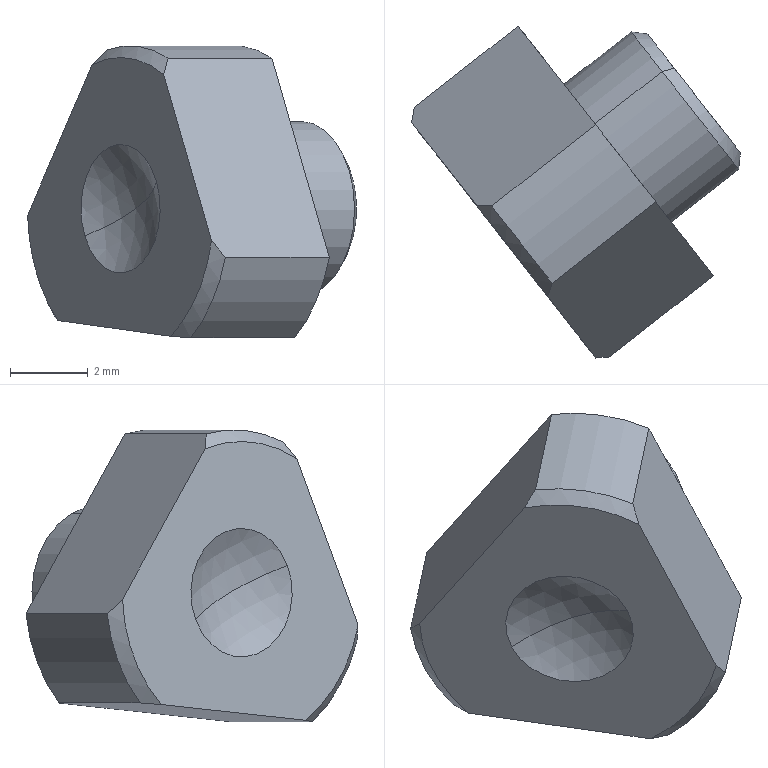Part | SolidWorks | features BaseBody 1 | 1 solid | 18 faces | box 8.485 x 8.562 x 7.531 mm | volume 194.109 mm3 | plane 6 | cylinder 5 | cone 5 | sphere 2 | commonest cylinder face diameters 8.4 x3 4.5 x2
STEP:
#1=CARTESIAN_POINT('',(-2.832,89.905,-119.788));
#2=VERTEX_POINT('',#1);
#3=CARTESIAN_POINT('',(-4.006,91.409,-115.712));
#4=VERTEX_POINT('',#3);
#5=CARTESIAN_POINT('',(-3.419,90.657,-117.75));
#6=DIRECTION('',(-0.788,-0.6157,0.));
#7=DIRECTION('',(-0.261,0.3341,0.9057));
#8=AXIS2_PLACEMENT_3D('',#5,#6,#7);
#9=CIRCLE('',#8,2.25);
#10=EDGE_CURVE('',#2,#4,#9,.T.);
#11=ORIENTED_EDGE('',*,*,#10,.T.);
#12=CARTESIAN_POINT('',(-5.74,90.054,-115.712));
#13=VERTEX_POINT('',#12);
#14=CARTESIAN_POINT('',(-8.656,87.776,-115.712));
#15=DIRECTION('',(-0.788,-0.6157,0.));
#16=VECTOR('',#15,1000.);
#17=LINE('',#14,#16);
#18=EDGE_CURVE('',#4,#13,#17,.T.);
#19=ORIENTED_EDGE('',*,*,#18,.T.);
#20=CARTESIAN_POINT('',(-4.565,88.551,-119.788));
#21=VERTEX_POINT('',#20);
#22=CARTESIAN_POINT('',(-5.153,89.303,-117.75));
#23=DIRECTION('',(-0.788,-0.6157,0.));
#24=DIRECTION('',(0.261,-0.3341,-0.9057));
#25=AXIS2_PLACEMENT_3D('',#22,#23,#24);
#26=CIRCLE('',#25,2.25);
#27=EDGE_CURVE('',#21,#13,#26,.T.);
#28=ORIENTED_EDGE('',*,*,#27,.F.);
#29=CARTESIAN_POINT('',(-7.481,86.273,-119.788));
#30=DIRECTION('',(-0.788,-0.6157,0.));
#31=VECTOR('',#30,1000.);
#32=LINE('',#29,#31);
#33=EDGE_CURVE('',#2,#21,#32,.T.);
#34=ORIENTED_EDGE('',*,*,#33,.F.);
#35=EDGE_LOOP('',(#11,#19,#28,#34));
#36=FACE_OUTER_BOUND('',#35,.T.);
#37=CARTESIAN_POINT('',(-8.068,87.025,-117.75));
#38=DIRECTION('',(-0.788,-0.6157,0.));
#39=DIRECTION('',(0.261,-0.3341,-0.9057));
#40=AXIS2_PLACEMENT_3D('',#37,#38,#39);
#41=CYLINDRICAL_SURFACE('',#40,2.25);
#42=ADVANCED_FACE('',(#36),#41,.T.);
#43=CARTESIAN_POINT('',(-7.674,87.332,-117.75));
#44=VERTEX_POINT('',#43);
#45=CARTESIAN_POINT('',(-7.144,85.841,-117.047));
#46=VERTEX_POINT('',#45);
#47=CARTESIAN_POINT('',(-10.038,85.485,-117.75));
#48=DIRECTION('',(0.261,-0.3341,-0.9057));
#49=DIRECTION('',(0.,0.9382,-0.3461));
#50=AXIS2_PLACEMENT_3D('',#47,#48,#49);
#51=CIRCLE('',#50,3.);
#52=EDGE_CURVE('',#44,#46,#51,.T.);
#53=ORIENTED_EDGE('',*,*,#52,.F.);
#54=CARTESIAN_POINT('',(-8.993,88.208,-118.453));
#55=VERTEX_POINT('',#54);
#56=CARTESIAN_POINT('',(-10.038,85.485,-117.75));
#57=DIRECTION('',(-0.261,0.3341,0.9057));
#58=DIRECTION('',(0.,-0.9382,0.3461));
#59=AXIS2_PLACEMENT_3D('',#56,#57,#58);
#60=CIRCLE('',#59,3.);
#61=EDGE_CURVE('',#44,#55,#60,.T.);
#62=ORIENTED_EDGE('',*,*,#61,.T.);
#63=CARTESIAN_POINT('',(-8.068,87.025,-117.75));
#64=DIRECTION('',(-0.788,-0.6157,0.));
#65=DIRECTION('',(0.261,-0.3341,-0.9057));
#66=AXIS2_PLACEMENT_3D('',#63,#64,#65);
#67=CIRCLE('',#66,1.658);
#68=EDGE_CURVE('',#55,#46,#67,.T.);
#69=ORIENTED_EDGE('',*,*,#68,.T.);
#70=EDGE_LOOP('',(#53,#62,#69));
#71=FACE_OUTER_BOUND('',#70,.T.);
#72=CARTESIAN_POINT('',(-10.038,85.485,-117.75));
#73=DIRECTION('',(-0.261,0.3341,0.9057));
#74=DIRECTION('',(0.5576,-0.7137,0.424));
#75=AXIS2_PLACEMENT_3D('',#72,#73,#74);
#76=SPHERICAL_SURFACE('',#75,3.);
#77=ADVANCED_FACE('',(#71),#76,.F.);
#78=CARTESIAN_POINT('',(-3.692,91.493,-115.984));
#79=VERTEX_POINT('',#78);
#80=CARTESIAN_POINT('',(-2.674,90.19,-119.516));
#81=VERTEX_POINT('',#80);
#82=CARTESIAN_POINT('',(-3.183,90.842,-117.75));
#83=DIRECTION('',(0.788,0.6157,0.));
#84=DIRECTION('',(-0.261,0.3341,0.9057));
#85=AXIS2_PLACEMENT_3D('',#82,#83,#84);
#86=CIRCLE('',#85,1.95);
#87=EDGE_CURVE('',#79,#81,#86,.T.);
#88=ORIENTED_EDGE('',*,*,#87,.F.);
#89=CARTESIAN_POINT('',(-4.006,91.409,-115.712));
#90=DIRECTION('',(-0.7418,-0.1991,0.6404));
#91=VECTOR('',#90,1000.);
#92=LINE('',#89,#91);
#93=EDGE_CURVE('',#79,#4,#92,.T.);
#94=ORIENTED_EDGE('',*,*,#93,.T.);
#95=ORIENTED_EDGE('',*,*,#10,.F.);
#96=CARTESIAN_POINT('',(-2.832,89.905,-119.788));
#97=DIRECTION('',(-0.3726,-0.6716,-0.6404));
#98=VECTOR('',#97,1000.);
#99=LINE('',#96,#98);
#100=EDGE_CURVE('',#81,#2,#99,.T.);
#101=ORIENTED_EDGE('',*,*,#100,.F.);
#102=EDGE_LOOP('',(#88,#94,#95,#101));
#103=FACE_OUTER_BOUND('',#102,.T.);
#104=CARTESIAN_POINT('',(-3.419,90.657,-117.75));
#105=DIRECTION('',(-0.788,-0.6157,0.));
#106=DIRECTION('',(0.261,-0.3341,-0.9057));
#107=AXIS2_PLACEMENT_3D('',#104,#105,#106);
#108=CONICAL_SURFACE('',#107,2.25,0.7854);
#109=ADVANCED_FACE('',(#103),#108,.T.);
#110=ORIENTED_EDGE('',*,*,#93,.F.);
#111=CARTESIAN_POINT('',(-3.183,90.842,-117.75));
#112=DIRECTION('',(0.788,0.6157,0.));
#113=DIRECTION('',(-0.261,0.3341,0.9057));
#114=AXIS2_PLACEMENT_3D('',#111,#112,#113);
#115=CIRCLE('',#114,1.95);
#116=EDGE_CURVE('',#81,#79,#115,.T.);
#117=ORIENTED_EDGE('',*,*,#116,.F.);
#118=ORIENTED_EDGE('',*,*,#100,.T.);
#119=CARTESIAN_POINT('',(-3.419,90.657,-117.75));
#120=DIRECTION('',(-0.788,-0.6157,0.));
#121=DIRECTION('',(-0.261,0.3341,0.9057));
#122=AXIS2_PLACEMENT_3D('',#119,#120,#121);
#123=CIRCLE('',#122,2.25);
#124=EDGE_CURVE('',#4,#2,#123,.T.);
#125=ORIENTED_EDGE('',*,*,#124,.F.);
#126=EDGE_LOOP('',(#110,#117,#118,#125));
#127=FACE_OUTER_BOUND('',#126,.T.);
#128=CARTESIAN_POINT('',(-3.419,90.657,-117.75));
#129=DIRECTION('',(-0.788,-0.6157,0.));
#130=DIRECTION('',(0.261,-0.3341,-0.9057));
#131=AXIS2_PLACEMENT_3D('',#128,#129,#130);
#132=CONICAL_SURFACE('',#131,2.25,0.7854);
#133=ADVANCED_FACE('',(#127),#132,.T.);
#134=CARTESIAN_POINT('',(-6.257,85.194,-121.081));
#135=VERTEX_POINT('',#134);
#136=CARTESIAN_POINT('',(-6.78,85.376,-121.041));
#137=VERTEX_POINT('',#136);
#138=CARTESIAN_POINT('',(-6.257,85.194,-121.081));
#139=CARTESIAN_POINT('',(-6.433,85.251,-121.068));
#140=CARTESIAN_POINT('',(-6.608,85.311,-121.055));
#141=CARTESIAN_POINT('',(-6.78,85.376,-121.041));
#142=B_SPLINE_CURVE_WITH_KNOTS('',3,(#138,#139,#140,#141),.UNSPECIFIED.,.F.,.F.,(4,4),(0.,1.),.UNSPECIFIED.);
#143=EDGE_CURVE('',#135,#137,#142,.T.);
#144=ORIENTED_EDGE('',*,*,#143,.F.);
#145=CARTESIAN_POINT('',(-5.364,84.05,-119.002));
#146=VERTEX_POINT('',#145);
#147=CARTESIAN_POINT('',(-7.832,87.209,-117.75));
#148=DIRECTION('',(0.788,0.6157,0.));
#149=DIRECTION('',(0.261,-0.3341,-0.9057));
#150=AXIS2_PLACEMENT_3D('',#147,#148,#149);
#151=CIRCLE('',#150,4.2);
#152=EDGE_CURVE('',#146,#135,#151,.T.);
#153=ORIENTED_EDGE('',*,*,#152,.F.);
#154=CARTESIAN_POINT('',(-5.722,84.022,-118.579));
#155=VERTEX_POINT('',#154);
#156=CARTESIAN_POINT('',(-5.722,84.022,-118.579));
#157=CARTESIAN_POINT('',(-5.605,84.028,-118.722));
#158=CARTESIAN_POINT('',(-5.485,84.038,-118.863));
#159=CARTESIAN_POINT('',(-5.364,84.05,-119.002));
#160=B_SPLINE_CURVE_WITH_KNOTS('',3,(#156,#157,#158,#159),.UNSPECIFIED.,.F.,.F.,(4,4),(0.,1.),.UNSPECIFIED.);
#161=EDGE_CURVE('',#155,#146,#160,.T.);
#162=ORIENTED_EDGE('',*,*,#161,.F.);
#163=CARTESIAN_POINT('',(-8.068,87.025,-117.75));
#164=DIRECTION('',(-0.788,-0.6157,0.));
#165=DIRECTION('',(0.261,-0.3341,-0.9057));
#166=AXIS2_PLACEMENT_3D('',#163,#164,#165);
#167=CIRCLE('',#166,3.9);
#168=EDGE_CURVE('',#137,#155,#167,.T.);
#169=ORIENTED_EDGE('',*,*,#168,.F.);
#170=EDGE_LOOP('',(#144,#153,#162,#169));
#171=FACE_OUTER_BOUND('',#170,.T.);
#172=CARTESIAN_POINT('',(-8.068,87.025,-117.75));
#173=DIRECTION('',(0.788,0.6157,0.));
#174=DIRECTION('',(-0.261,0.3341,0.9057));
#175=AXIS2_PLACEMENT_3D('',#172,#173,#174);
#176=CONICAL_SURFACE('',#175,3.9,0.7854);
#177=ADVANCED_FACE('',(#171),#176,.T.);
#178=CARTESIAN_POINT('',(-10.395,90.491,-118.299));
#179=VERTEX_POINT('',#178);
#180=CARTESIAN_POINT('',(-10.467,90.095,-117.916));
#181=VERTEX_POINT('',#180);
#182=CARTESIAN_POINT('',(-10.395,90.491,-118.299));
#183=CARTESIAN_POINT('',(-10.423,90.358,-118.174));
#184=CARTESIAN_POINT('',(-10.447,90.226,-118.046));
#185=CARTESIAN_POINT('',(-10.467,90.095,-117.916));
#186=B_SPLINE_CURVE_WITH_KNOTS('',3,(#182,#183,#184,#185),.UNSPECIFIED.,.F.,.F.,(4,4),(0.,1.),.UNSPECIFIED.);
#187=EDGE_CURVE('',#179,#181,#186,.T.);
#188=ORIENTED_EDGE('',*,*,#187,.F.);
#189=CARTESIAN_POINT('',(-9.734,89.643,-120.596));
#190=VERTEX_POINT('',#189);
#191=CARTESIAN_POINT('',(-7.832,87.209,-117.75));
#192=DIRECTION('',(0.788,0.6157,0.));
#193=DIRECTION('',(0.261,-0.3341,-0.9057));
#194=AXIS2_PLACEMENT_3D('',#191,#192,#193);
#195=CIRCLE('',#194,4.2);
#196=EDGE_CURVE('',#190,#179,#195,.T.);
#197=ORIENTED_EDGE('',*,*,#196,.F.);
#198=CARTESIAN_POINT('',(-9.683,89.092,-120.636));
#199=VERTEX_POINT('',#198);
#200=CARTESIAN_POINT('',(-9.683,89.092,-120.636));
#201=CARTESIAN_POINT('',(-9.705,89.275,-120.622));
#202=CARTESIAN_POINT('',(-9.721,89.459,-120.609));
#203=CARTESIAN_POINT('',(-9.734,89.643,-120.596));
#204=B_SPLINE_CURVE_WITH_KNOTS('',3,(#200,#201,#202,#203),.UNSPECIFIED.,.F.,.F.,(4,4),(0.,1.),.UNSPECIFIED.);
#205=EDGE_CURVE('',#199,#190,#204,.T.);
#206=ORIENTED_EDGE('',*,*,#205,.F.);
#207=CARTESIAN_POINT('',(-8.068,87.025,-117.75));
#208=DIRECTION('',(-0.788,-0.6157,0.));
#209=DIRECTION('',(0.261,-0.3341,-0.9057));
#210=AXIS2_PLACEMENT_3D('',#207,#208,#209);
#211=CIRCLE('',#210,3.9);
#212=EDGE_CURVE('',#181,#199,#211,.T.);
#213=ORIENTED_EDGE('',*,*,#212,.F.);
#214=EDGE_LOOP('',(#188,#197,#206,#213));
#215=FACE_OUTER_BOUND('',#214,.T.);
#216=CARTESIAN_POINT('',(-8.068,87.025,-117.75));
#217=DIRECTION('',(0.788,0.6157,0.));
#218=DIRECTION('',(-0.261,0.3341,0.9057));
#219=AXIS2_PLACEMENT_3D('',#216,#217,#218);
#220=CONICAL_SURFACE('',#219,3.9,0.7854);
#221=ADVANCED_FACE('',(#215),#220,.T.);
#222=CARTESIAN_POINT('',(-6.843,85.944,-113.869));
#223=VERTEX_POINT('',#222);
#224=CARTESIAN_POINT('',(-6.957,85.603,-114.292));
#225=VERTEX_POINT('',#224);
#226=CARTESIAN_POINT('',(-6.843,85.944,-113.869));
#227=CARTESIAN_POINT('',(-6.885,85.829,-114.008));
#228=CARTESIAN_POINT('',(-6.923,85.715,-114.149));
#229=CARTESIAN_POINT('',(-6.957,85.603,-114.292));
#230=B_SPLINE_CURVE_WITH_KNOTS('',3,(#226,#227,#228,#229),.UNSPECIFIED.,.F.,.F.,(4,4),(0.,1.),.UNSPECIFIED.);
#231=EDGE_CURVE('',#223,#225,#230,.T.);
#232=ORIENTED_EDGE('',*,*,#231,.F.);
#233=CARTESIAN_POINT('',(-8.398,87.934,-113.652));
#234=VERTEX_POINT('',#233);
#235=CARTESIAN_POINT('',(-7.832,87.209,-117.75));
#236=DIRECTION('',(0.788,0.6157,0.));
#237=DIRECTION('',(0.261,-0.3341,-0.9057));
#238=AXIS2_PLACEMENT_3D('',#235,#236,#237);
#239=CIRCLE('',#238,4.2);
#240=EDGE_CURVE('',#234,#223,#239,.T.);
#241=ORIENTED_EDGE('',*,*,#240,.F.);
#242=CARTESIAN_POINT('',(-8.799,87.96,-114.035));
#243=VERTEX_POINT('',#242);
#244=CARTESIAN_POINT('',(-8.799,87.96,-114.035));
#245=CARTESIAN_POINT('',(-8.668,87.948,-113.905));
#246=CARTESIAN_POINT('',(-8.534,87.94,-113.778));
#247=CARTESIAN_POINT('',(-8.398,87.934,-113.652));
#248=B_SPLINE_CURVE_WITH_KNOTS('',3,(#244,#245,#246,#247),.UNSPECIFIED.,.F.,.F.,(4,4),(0.,1.),.UNSPECIFIED.);
#249=EDGE_CURVE('',#243,#234,#248,.T.);
#250=ORIENTED_EDGE('',*,*,#249,.F.);
#251=CARTESIAN_POINT('',(-8.068,87.025,-117.75));
#252=DIRECTION('',(-0.788,-0.6157,0.));
#253=DIRECTION('',(0.261,-0.3341,-0.9057));
#254=AXIS2_PLACEMENT_3D('',#251,#252,#253);
#255=CIRCLE('',#254,3.9);
#256=EDGE_CURVE('',#225,#243,#255,.T.);
#257=ORIENTED_EDGE('',*,*,#256,.F.);
#258=EDGE_LOOP('',(#232,#241,#250,#257));
#259=FACE_OUTER_BOUND('',#258,.T.);
#260=CARTESIAN_POINT('',(-8.068,87.025,-117.75));
#261=DIRECTION('',(0.788,0.6157,0.));
#262=DIRECTION('',(-0.261,0.3341,0.9057));
#263=AXIS2_PLACEMENT_3D('',#260,#261,#262);
#264=CONICAL_SURFACE('',#263,3.9,0.7854);
#265=ADVANCED_FACE('',(#259),#264,.T.);
#266=CARTESIAN_POINT('',(-10.632,90.306,-118.299));
#267=DIRECTION('',(0.3524,-0.451,0.82));
#268=VECTOR('',#267,1000.);
#269=LINE('',#266,#268);
#270=EDGE_CURVE('',#181,#243,#269,.T.);
#271=ORIENTED_EDGE('',*,*,#270,.T.);
#272=ORIENTED_EDGE('',*,*,#249,.T.);
#273=CARTESIAN_POINT('',(-5.719,90.028,-113.652));
#274=VERTEX_POINT('',#273);
#275=CARTESIAN_POINT('',(-3.749,91.567,-113.652));
#276=DIRECTION('',(-0.788,-0.6157,0.));
#277=VECTOR('',#276,1000.);
#278=LINE('',#275,#277);
#279=EDGE_CURVE('',#274,#234,#278,.T.);
#280=ORIENTED_EDGE('',*,*,#279,.F.);
#281=CARTESIAN_POINT('',(-7.716,92.584,-118.299));
#282=VERTEX_POINT('',#281);
#283=CARTESIAN_POINT('',(-5.436,89.665,-112.993));
#284=DIRECTION('',(-0.3524,0.451,-0.82));
#285=VECTOR('',#284,1000.);
#286=LINE('',#283,#285);
#287=EDGE_CURVE('',#274,#282,#286,.T.);
#288=ORIENTED_EDGE('',*,*,#287,.T.);
#289=CARTESIAN_POINT('',(-5.746,94.123,-118.299));
#290=DIRECTION('',(-0.788,-0.6157,0.));
#291=VECTOR('',#290,1000.);
#292=LINE('',#289,#291);
#293=EDGE_CURVE('',#282,#179,#292,.T.);
#294=ORIENTED_EDGE('',*,*,#293,.T.);
#295=ORIENTED_EDGE('',*,*,#187,.T.);
#296=EDGE_LOOP('',(#271,#272,#280,#288,#294,#295));
#297=FACE_OUTER_BOUND('',#296,.T.);
#298=CARTESIAN_POINT('',(-5.746,94.123,-118.299));
#299=DIRECTION('',(0.5048,-0.6462,-0.5724));
#300=DIRECTION('',(0.,0.6631,-0.7486));
#301=AXIS2_PLACEMENT_3D('',#298,#299,#300);
#302=PLANE('',#301);
#303=ADVANCED_FACE('',(#297),#302,.F.);
#304=CARTESIAN_POINT('',(-6.494,85.009,-121.081));
#305=DIRECTION('',(-0.6134,0.7851,0.08568));
#306=VECTOR('',#305,1000.);
#307=LINE('',#304,#306);
#308=EDGE_CURVE('',#137,#199,#307,.T.);
#309=ORIENTED_EDGE('',*,*,#308,.T.);
#310=ORIENTED_EDGE('',*,*,#205,.T.);
#311=CARTESIAN_POINT('',(-7.054,91.737,-120.596));
#312=VERTEX_POINT('',#311);
#313=CARTESIAN_POINT('',(-5.084,93.276,-120.596));
#314=DIRECTION('',(-0.788,-0.6157,0.));
#315=VECTOR('',#314,1000.);
#316=LINE('',#313,#315);
#317=EDGE_CURVE('',#312,#190,#316,.T.);
#318=ORIENTED_EDGE('',*,*,#317,.F.);
#319=CARTESIAN_POINT('',(-3.578,87.287,-121.081));
#320=VERTEX_POINT('',#319);
#321=CARTESIAN_POINT('',(-3.085,86.656,-121.15));
#322=DIRECTION('',(0.6134,-0.7851,-0.08568));
#323=VECTOR('',#322,1000.);
#324=LINE('',#321,#323);
#325=EDGE_CURVE('',#312,#320,#324,.T.);
#326=ORIENTED_EDGE('',*,*,#325,.T.);
#327=CARTESIAN_POINT('',(-1.608,88.826,-121.081));
#328=DIRECTION('',(-0.788,-0.6157,0.));
#329=VECTOR('',#328,1000.);
#330=LINE('',#327,#329);
#331=EDGE_CURVE('',#320,#135,#330,.T.);
#332=ORIENTED_EDGE('',*,*,#331,.T.);
#333=ORIENTED_EDGE('',*,*,#143,.T.);
#334=EDGE_LOOP('',(#309,#310,#318,#326,#332,#333));
#335=FACE_OUTER_BOUND('',#334,.T.);
#336=CARTESIAN_POINT('',(-1.608,88.826,-121.081));
#337=DIRECTION('',(0.05275,-0.06752,0.9963));
#338=DIRECTION('',(-0.788,-0.6157,0.));
#339=AXIS2_PLACEMENT_3D('',#336,#337,#338);
#340=PLANE('',#339);
#341=ADVANCED_FACE('',(#335),#340,.F.);
#342=CARTESIAN_POINT('',(-4.164,88.037,-113.869));
#343=VERTEX_POINT('',#342);
#344=CARTESIAN_POINT('',(-2.194,89.576,-113.869));
#345=DIRECTION('',(-0.788,-0.6157,0.));
#346=VECTOR('',#345,1000.);
#347=LINE('',#344,#346);
#348=EDGE_CURVE('',#343,#223,#347,.T.);
#349=ORIENTED_EDGE('',*,*,#348,.T.);
#350=ORIENTED_EDGE('',*,*,#231,.T.);
#351=CARTESIAN_POINT('',(-7.079,85.759,-113.869));
#352=DIRECTION('',(0.261,-0.3341,-0.9057));
#353=VECTOR('',#352,1000.);
#354=LINE('',#351,#353);
#355=EDGE_CURVE('',#225,#155,#354,.T.);
#356=ORIENTED_EDGE('',*,*,#355,.T.);
#357=ORIENTED_EDGE('',*,*,#161,.T.);
#358=CARTESIAN_POINT('',(-2.684,86.143,-119.002));
#359=VERTEX_POINT('',#358);
#360=CARTESIAN_POINT('',(-0.7145,87.683,-119.002));
#361=DIRECTION('',(-0.788,-0.6157,0.));
#362=VECTOR('',#361,1000.);
#363=LINE('',#360,#362);
#364=EDGE_CURVE('',#359,#146,#363,.T.);
#365=ORIENTED_EDGE('',*,*,#364,.F.);
#366=CARTESIAN_POINT('',(-3.424,87.09,-116.436));
#367=DIRECTION('',(-0.261,0.3341,0.9057));
#368=VECTOR('',#367,1000.);
#369=LINE('',#366,#368);
#370=EDGE_CURVE('',#359,#343,#369,.T.);
#371=ORIENTED_EDGE('',*,*,#370,.T.);
#372=EDGE_LOOP('',(#349,#350,#356,#357,#365,#371));
#373=FACE_OUTER_BOUND('',#372,.T.);
#374=CARTESIAN_POINT('',(-2.194,89.576,-113.869));
#375=DIRECTION('',(-0.5576,0.7137,-0.424));
#376=DIRECTION('',(-0.6053,0.,0.796));
#377=AXIS2_PLACEMENT_3D('',#374,#375,#376);
#378=PLANE('',#377);
#379=ADVANCED_FACE('',(#373),#378,.F.);
#380=CARTESIAN_POINT('',(-8.068,87.025,-117.75));
#381=DIRECTION('',(-0.788,-0.6157,0.));
#382=DIRECTION('',(0.261,-0.3341,-0.9057));
#383=AXIS2_PLACEMENT_3D('',#380,#381,#382);
#384=CIRCLE('',#383,1.658);
#385=EDGE_CURVE('',#46,#55,#384,.T.);
#386=ORIENTED_EDGE('',*,*,#385,.F.);
#387=ORIENTED_EDGE('',*,*,#68,.F.);
#388=EDGE_LOOP('',(#386,#387));
#389=FACE_BOUND('',#388,.T.);
#390=ORIENTED_EDGE('',*,*,#355,.F.);
#391=ORIENTED_EDGE('',*,*,#256,.T.);
#392=ORIENTED_EDGE('',*,*,#270,.F.);
#393=ORIENTED_EDGE('',*,*,#212,.T.);
#394=ORIENTED_EDGE('',*,*,#308,.F.);
#395=ORIENTED_EDGE('',*,*,#168,.T.);
#396=EDGE_LOOP('',(#390,#391,#392,#393,#394,#395));
#397=FACE_OUTER_BOUND('',#396,.T.);
#398=CARTESIAN_POINT('',(-7.144,85.841,-117.047));
#399=DIRECTION('',(-0.788,-0.6157,0.));
#400=DIRECTION('',(-0.6157,0.788,0.));
#401=AXIS2_PLACEMENT_3D('',#398,#399,#400);
#402=PLANE('',#401);
#403=ADVANCED_FACE('',(#389,#397),#402,.T.);
#404=ORIENTED_EDGE('',*,*,#61,.F.);
#405=ORIENTED_EDGE('',*,*,#52,.T.);
#406=ORIENTED_EDGE('',*,*,#385,.T.);
#407=EDGE_LOOP('',(#404,#405,#406));
#408=FACE_OUTER_BOUND('',#407,.T.);
#409=CARTESIAN_POINT('',(-10.038,85.485,-117.75));
#410=DIRECTION('',(-0.261,0.3341,0.9057));
#411=DIRECTION('',(0.5576,-0.7137,0.424));
#412=AXIS2_PLACEMENT_3D('',#409,#410,#411);
#413=SPHERICAL_SURFACE('',#412,3.);
#414=ADVANCED_FACE('',(#408),#413,.F.);
#415=ORIENTED_EDGE('',*,*,#116,.T.);
#416=ORIENTED_EDGE('',*,*,#87,.T.);
#417=EDGE_LOOP('',(#415,#416));
#418=FACE_OUTER_BOUND('',#417,.T.);
#419=CARTESIAN_POINT('',(-1.928,89.236,-116.796));
#420=DIRECTION('',(0.788,0.6157,0.));
#421=DIRECTION('',(0.,0.,-1.));
#422=AXIS2_PLACEMENT_3D('',#419,#420,#421);
#423=PLANE('',#422);
#424=ADVANCED_FACE('',(#418),#423,.T.);
#425=ORIENTED_EDGE('',*,*,#18,.F.);
#426=ORIENTED_EDGE('',*,*,#124,.T.);
#427=ORIENTED_EDGE('',*,*,#33,.T.);
#428=CARTESIAN_POINT('',(-5.153,89.303,-117.75));
#429=DIRECTION('',(-0.788,-0.6157,0.));
#430=DIRECTION('',(0.261,-0.3341,-0.9057));
#431=AXIS2_PLACEMENT_3D('',#428,#429,#430);
#432=CIRCLE('',#431,2.25);
#433=EDGE_CURVE('',#13,#21,#432,.T.);
#434=ORIENTED_EDGE('',*,*,#433,.F.);
#435=EDGE_LOOP('',(#425,#426,#427,#434));
#436=FACE_OUTER_BOUND('',#435,.T.);
#437=CARTESIAN_POINT('',(-8.068,87.025,-117.75));
#438=DIRECTION('',(-0.788,-0.6157,0.));
#439=DIRECTION('',(0.261,-0.3341,-0.9057));
#440=AXIS2_PLACEMENT_3D('',#437,#438,#439);
#441=CYLINDRICAL_SURFACE('',#440,2.25);
#442=ADVANCED_FACE('',(#436),#441,.T.);
#443=ORIENTED_EDGE('',*,*,#27,.T.);
#444=ORIENTED_EDGE('',*,*,#433,.T.);
#445=EDGE_LOOP('',(#443,#444));
#446=FACE_BOUND('',#445,.T.);
#447=ORIENTED_EDGE('',*,*,#287,.F.);
#448=CARTESIAN_POINT('',(-5.153,89.303,-117.75));
#449=DIRECTION('',(-0.788,-0.6157,0.));
#450=DIRECTION('',(0.261,-0.3341,-0.9057));
#451=AXIS2_PLACEMENT_3D('',#448,#449,#450);
#452=CIRCLE('',#451,4.2);
#453=EDGE_CURVE('',#343,#274,#452,.T.);
#454=ORIENTED_EDGE('',*,*,#453,.F.);
#455=ORIENTED_EDGE('',*,*,#370,.F.);
#456=CARTESIAN_POINT('',(-5.153,89.303,-117.75));
#457=DIRECTION('',(-0.788,-0.6157,0.));
#458=DIRECTION('',(0.261,-0.3341,-0.9057));
#459=AXIS2_PLACEMENT_3D('',#456,#457,#458);
#460=CIRCLE('',#459,4.2);
#461=EDGE_CURVE('',#320,#359,#460,.T.);
#462=ORIENTED_EDGE('',*,*,#461,.F.);
#463=ORIENTED_EDGE('',*,*,#325,.F.);
#464=CARTESIAN_POINT('',(-5.153,89.303,-117.75));
#465=DIRECTION('',(-0.788,-0.6157,0.));
#466=DIRECTION('',(0.261,-0.3341,-0.9057));
#467=AXIS2_PLACEMENT_3D('',#464,#465,#466);
#468=CIRCLE('',#467,4.2);
#469=EDGE_CURVE('',#282,#312,#468,.T.);
#470=ORIENTED_EDGE('',*,*,#469,.F.);
#471=EDGE_LOOP('',(#447,#454,#455,#462,#463,#470));
#472=FACE_OUTER_BOUND('',#471,.T.);
#473=CARTESIAN_POINT('',(-2.811,86.305,-115.969));
#474=DIRECTION('',(0.788,0.6157,0.));
#475=DIRECTION('',(0.,0.,-1.));
#476=AXIS2_PLACEMENT_3D('',#473,#474,#475);
#477=PLANE('',#476);
#478=ADVANCED_FACE('',(#446,#472),#477,.T.);
#479=ORIENTED_EDGE('',*,*,#364,.T.);
#480=ORIENTED_EDGE('',*,*,#152,.T.);
#481=ORIENTED_EDGE('',*,*,#331,.F.);
#482=ORIENTED_EDGE('',*,*,#461,.T.);
#483=EDGE_LOOP('',(#479,#480,#481,#482));
#484=FACE_OUTER_BOUND('',#483,.T.);
#485=CARTESIAN_POINT('',(-8.068,87.025,-117.75));
#486=DIRECTION('',(-0.788,-0.6157,0.));
#487=DIRECTION('',(0.261,-0.3341,-0.9057));
#488=AXIS2_PLACEMENT_3D('',#485,#486,#487);
#489=CYLINDRICAL_SURFACE('',#488,4.2);
#490=ADVANCED_FACE('',(#484),#489,.T.);
#491=ORIENTED_EDGE('',*,*,#317,.T.);
#492=ORIENTED_EDGE('',*,*,#196,.T.);
#493=ORIENTED_EDGE('',*,*,#293,.F.);
#494=ORIENTED_EDGE('',*,*,#469,.T.);
#495=EDGE_LOOP('',(#491,#492,#493,#494));
#496=FACE_OUTER_BOUND('',#495,.T.);
#497=CARTESIAN_POINT('',(-8.068,87.025,-117.75));
#498=DIRECTION('',(-0.788,-0.6157,0.));
#499=DIRECTION('',(0.261,-0.3341,-0.9057));
#500=AXIS2_PLACEMENT_3D('',#497,#498,#499);
#501=CYLINDRICAL_SURFACE('',#500,4.2);
#502=ADVANCED_FACE('',(#496),#501,.T.);
#503=ORIENTED_EDGE('',*,*,#279,.T.);
#504=ORIENTED_EDGE('',*,*,#240,.T.);
#505=ORIENTED_EDGE('',*,*,#348,.F.);
#506=ORIENTED_EDGE('',*,*,#453,.T.);
#507=EDGE_LOOP('',(#503,#504,#505,#506));
#508=FACE_OUTER_BOUND('',#507,.T.);
#509=CARTESIAN_POINT('',(-8.068,87.025,-117.75));
#510=DIRECTION('',(-0.788,-0.6157,0.));
#511=DIRECTION('',(0.261,-0.3341,-0.9057));
#512=AXIS2_PLACEMENT_3D('',#509,#510,#511);
#513=CYLINDRICAL_SURFACE('',#512,4.2);
#514=ADVANCED_FACE('',(#508),#513,.T.);
#515=CLOSED_SHELL('',(#42,#77,#109,#133,#177,#221,#265,#303,#341,#379,#403,#414,#424,#442,#478,#490,#502,#514));
#516=MANIFOLD_SOLID_BREP('',#515);
#517=CARTESIAN_POINT('',(0.,0.,0.));
#518=DIRECTION('',(0.,0.,1.));
#519=DIRECTION('',(1.,0.,0.));
#520=AXIS2_PLACEMENT_3D('',#517,#518,#519);
#521=(LENGTH_UNIT()NAMED_UNIT(*)SI_UNIT(.MILLI.,.METRE.));
#522=UNCERTAINTY_MEASURE_WITH_UNIT(LENGTH_MEASURE(0.00001),#521,'','');
#523=(NAMED_UNIT(*)PLANE_ANGLE_UNIT()SI_UNIT($,.RADIAN.));
#524=(NAMED_UNIT(*)SI_UNIT($,.STERADIAN.)SOLID_ANGLE_UNIT());
#525=(GEOMETRIC_REPRESENTATION_CONTEXT(3)GLOBAL_UNCERTAINTY_ASSIGNED_CONTEXT((#522))GLOBAL_UNIT_ASSIGNED_CONTEXT((#521,#523,#524))REPRESENTATION_CONTEXT('',''));
#526=ADVANCED_BREP_SHAPE_REPRESENTATION('',(#516,#520),#525);